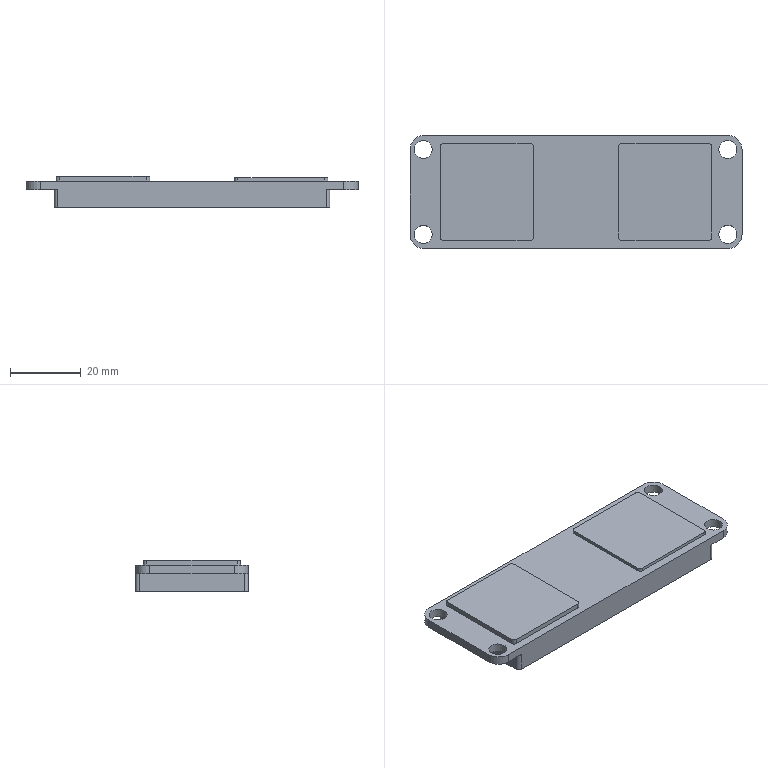NC program | NX | posted with a generic post | part box 94 x 32 x 9 mm
Whole program:
N10 G17 G21 G94 G90
(101_COPY , TOOL : D50-120)
N12 T01 M6
N14 G54
N16 G17 G0 G90 X-97. Y-1.5 S3000 M3
N18 G43 Z49.5 H1
N20 Z6.171
N22 G94 G1 Z5.671 F3000.
N24 X-72.
N26 X72.
N28 X97.
N30 Z6.171
N32 G0 Z49.5
N34 X-97.
N36 Z5.243
N38 G1 Z4.743
N40 X-72.
N42 X72.
N44 X97.
N46 Z5.243
N48 G0 Z49.5
N50 X-97.
N52 Z4.314
N54 G1 Z3.814
N56 X-72.
N58 X72.
N60 X97.
N62 Z4.314
N64 G0 Z49.5
N66 X-97.
N68 Z3.386
N70 G1 Z2.886
N72 X-72.
N74 X72.
N76 X97.
N78 Z3.386
N80 G0 Z49.5
N82 X-97.
N84 Z2.457
N86 G1 Z1.957
N88 X-72.
N90 X72.
N92 X97.
N94 Z2.457
N96 G0 Z49.5
N98 X-97.
N100 Z1.529
N102 G1 Z1.029
N104 X-72.
N106 X72.
N108 X97.
N110 Z1.529
N112 G0 Z49.5
N114 X-97.
N116 Z0.6
N118 G1 Z0.1
N120 X-72.
N122 X72.
N124 X97.
N126 Z0.6
N128 G0 Z49.5
N130 M5
(1013 , TOOL : ER25-D10-20)
N132 T02 M6
N134 G54
N136 G17 G0 G90 X-4.07 Y26. S5000 M3
N138 G43 Z49.5 H2
N140 Z1.7
N142 G94 G1 Z-1.3 F2000.
N144 X-0.713 Y21.
N146 G2 X0. Y19.824 R14.8
N148 X0.713 Y21. R14.8
N150 G1 X4.07 Y26.
N152 Z1.7
N154 G0 Z49.5
N156 Y-26.
N158 Z1.7
N160 G1 Z-1.3
N162 X0.713 Y-21.
N164 G2 X0. Y-19.824 R14.8
N166 G1 X-1.976 Y-15.231
N168 G3 X-1.7 Y-12.75 R11.3
N170 G1 Y12.75
N172 G3 X-1.976 Y15.231 R11.3
N174 X1.976 Y15.231 R5.
N176 X1.7 Y12.75 R11.3
N178 G1 Y-12.75
N180 G3 X1.976 Y-15.231 R11.3
N182 X-1.976 Y-15.231 R5.
N184 G1 X0. Y-19.824
N186 G2 X-0.713 Y-21. R14.8
N188 G1 X-7.77 Y-16.262
N190 G2 X-13. Y-19.05 R6.3
N192 G1 X-37.5
N194 G2 X-43.8 Y-12.75 R6.3
N196 G1 Y12.75
N198 G2 X-37.5 Y19.05 R6.3
N200 G1 X-13.
N202 G2 X-6.7 Y12.75 R6.3
N204 G1 Y-12.75
N206 G2 X-7.77 Y-16.262 R6.3
N208 G1 Z1.7
N210 G0 Z49.5
N212 X1.7 Y-12.75
N214 Z1.7
N216 G1 Z-1.3
N218 X6.7
N220 Y12.75
N222 G2 X13. Y19.05 R6.3
N224 G1 X37.5
N226 G2 X43.8 Y12.75 R6.3
N228 G1 Y-12.75
N230 G2 X37.5 Y-19.05 R6.3
N232 G1 X13.
N234 G2 X6.7 Y-12.75 R6.3
N236 G1 X1.7
N238 Y-26.
N240 Z1.7
N242 G0 Z49.5
N244 M5
(1013_COPY , TOOL : ER25-D10-30_G)
N246 T10 M6
N248 G54
N250 G17 G0 G90 X48.5 Y-11.25 S5000 M3
N252 G43 Z49.5 H10
N254 Z2.5
N256 G94 G1 Z-0.5 F1000.
N258 X43.5
N260 X7.
N262 Y-3.75
N264 X43.5
N266 Y3.75
N268 X7.
N270 Y11.25
N272 X43.5
N274 X48.5
N276 Z2.5
N278 G0 Z49.5
N280 X-2. Y-11.25
N282 Z3.
N284 G1 Z0.
N286 X-7.
N288 X-43.5
N290 Y-3.75
N292 X-7.
N294 Y3.75
N296 X-43.5
N298 Y11.25
N300 X-7.
N302 X-2.
N304 Z3.
N306 G0 Z49.5
(1014 , TOOL : ER25-D10-30_G)
N308 X-1.742 Y33.489
N310 Z1.6
N312 G1 Z-1.4
N314 G2 X0.713 Y21. R9.
N316 G3 X0. Y19.824 R14.8
N318 X-0.713 Y21. R14.8
N320 G2 X1.742 Y33.489 R9.
N322 G1 Z1.6
N324 G0 Z49.5
N326 Y-33.489
N328 Z1.6
N330 G1 Z-1.4
N332 G2 X-0.713 Y-21. R9.
N334 G3 X0. Y-19.824 R14.8
N336 G1 X-1.976 Y-15.231
N338 G3 X-1.7 Y-12.75 R11.3
N340 G1 Y12.75
N342 G3 X-1.976 Y15.231 R11.3
N344 X1.976 Y15.231 R5.
N346 X1.7 Y12.75 R11.3
N348 G1 Y-12.75
N350 G3 X1.976 Y-15.231 R11.3
N352 X-1.976 Y-15.231 R5.
N354 G1 X0. Y-19.824
N356 G3 X0.713 Y-21. R14.8
N358 G1 X7.77 Y-16.262
N360 G2 X6.7 Y-12.75 R6.3
N362 G1 Y12.75
N364 G2 X13. Y19.05 R6.3
N366 G1 X37.5
N368 G2 X43.8 Y12.75 R6.3
N370 G1 Y-12.75
N372 G2 X37.5 Y-19.05 R6.3
N374 G1 X13.
N376 G2 X7.77 Y-16.262 R6.3
N378 G3 X-4.719 Y-13.807 R9.
N380 G1 Y-26.
N382 Z1.6
N384 G0 Z49.5
N386 X-53.047 Y-21.75
N388 Z1.6
N390 G1 Z-1.4
N392 X-52.8
N394 G3 X-43.8 Y-12.75 R9.
N396 G1 Y12.75
N398 G2 X-37.5 Y19.05 R6.3
N400 G1 X-13.
N402 G2 X-6.7 Y12.75 R6.3
N404 G1 Y-12.75
N406 G2 X-13. Y-19.05 R6.3
N408 G1 X-37.5
N410 G2 X-43.8 Y-12.75 R6.3
N412 G3 X-52.8 Y-3.75 R9.
N414 G1 X-57.
N416 Z1.6
N418 G0 Z49.5
(PLANAR_MILL_1_3 , TOOL : ER25-D10-30_G)
N420 X-47.8 Y-2.995
N422 G1 Z-0.9 F4500.
N424 Z-1.4 F1000.
N426 G41 X-47.5 Y-3. D10
N428 X-46.5
N430 G3 X-43.5 Y0. R3.
N432 G1 Y12.75
N434 G2 X-37.5 Y18.75 R6.
N436 G1 X-13.
N438 G2 X-7. Y12.75 R6.
N440 G1 Y-12.75
N442 G2 X-13. Y-18.75 R6.
N444 G1 X-37.5
N446 G2 X-43.5 Y-12.75 R6.
N448 G1 Y0.
N450 Y0.5
N452 G3 X-46.5 Y3.5 R3.
N454 G1 X-47.5
N456 G40
N458 X-47.8 Y3.495
N460 Z-0.9
N462 G0 Z0.5
N464 G1 X28.245 Y-23.05 F6000.
N466 Z-0.9 F4500.
N468 Z-1.4 F1000.
N470 G41 X28.25 Y-22.75
N472 Y-21.75
N474 G3 X25.25 Y-18.75 R3.
N476 G1 X13.
N478 G2 X7. Y-12.75 R6.
N480 G1 Y12.75
N482 G2 X13. Y18.75 R6.
N484 G1 X37.5
N486 G2 X43.5 Y12.75 R6.
N488 G1 Y-12.75
N490 G2 X37.5 Y-18.75 R6.
N492 G1 X25.25
N494 X24.75
N496 G3 X21.75 Y-21.75 R3.
N498 G1 Y-22.75
N500 G40
N502 X21.755 Y-23.05
N504 Z-0.9
N506 G0 Z49.5
N508 M5
(1015 , TOOL : Φ3倒角刀)
N510 T06 M6
N512 G54
N514 G17 G0 G90 X-40.9 Y-0.895 S5000 M3
N516 G43 Z49.5 H6
N518 G94 G1 Z-0.5 F4500.
N520 Z-1. F1000.
N522 G41 X-40.6 Y-0.9 D6
N524 X-40.3
N526 G3 X-39.4 Y0. R0.9
N528 G1 Y12.75
N530 G2 X-37.5 Y14.65 R1.9
N532 G1 X-13.
N534 G2 X-11.1 Y12.75 R1.9
N536 G1 Y-12.75
N538 G2 X-13. Y-14.65 R1.9
N540 G1 X-37.5
N542 G2 X-39.4 Y-12.75 R1.9
N544 G1 Y0.
N546 Y0.5
N548 G3 X-40.3 Y1.4 R0.9
N550 G1 X-40.6
N552 G40
N554 X-40.9 Y1.395
N556 Z-0.5
N558 G0 Z0.5
N560 G1 X26.145 Y-15.65 F6000.
N562 Z-0.5 F4500.
N564 Z-1. F1000.
N566 G41 X26.15 Y-15.35
N568 Y-15.05
N570 G3 X25.25 Y-14.15 R0.9
N572 G1 X13.
N574 G2 X11.6 Y-12.75 R1.4
N576 G1 Y12.75
N578 G2 X13. Y14.15 R1.4
N580 G1 X37.5
N582 G2 X38.9 Y12.75 R1.4
N584 G1 Y-12.75
N586 G2 X37.5 Y-14.15 R1.4
N588 G1 X25.25
N590 X24.75
N592 G3 X23.85 Y-15.05 R0.9
N594 G1 Y-15.35
N596 G40
N598 X23.855 Y-15.65
N600 Z-0.5
N602 G0 Z49.5
(PLANAR_MILL_1_3_COPY_COPY , TOOL : Φ3倒角刀)
N604 X-0.895 Y18.4
N606 G1 Z-1.9 F4500.
N608 Z-2.4 F1000.
N610 G41 X-0.9 Y18.1
N612 Y17.8
N614 G3 X0. Y16.9 R0.9
N616 G1 X43.
N618 G2 X47.9 Y12. R4.9
N620 G1 Y-12.
N622 G2 X43. Y-16.9 R4.9
N624 G1 X-43.
N626 G2 X-47.9 Y-12. R4.9
N628 G1 Y12.
N630 G2 X-43. Y16.9 R4.9
N632 G1 X0.
N634 X0.5
N636 G3 X1.4 Y17.8 R0.9
N638 G1 Y18.1
N640 G40
N642 X1.395 Y18.4
N644 Z-1.9
N646 G0 Z49.5
(PLANAR_MILL_1_3_COPY_COPY_COPY , TOOL : Φ3倒角刀)
N648 X-43.538 Y-11.654
N650 G1 Z-1.9 F4500.
N652 Z-2.4 F1000.
N654 G41 X-44. Y-11.1
N656 G3 X-44.9 Y-12. R0.9
N658 X-43.25 Y-13.65 R1.65
N660 X-44.9 Y-12. R-1.65
N662 X-44.825 Y-12.492 R1.65
N664 X-43.697 Y-13.083 R0.9
N666 G40
N668 G1 X-43.422 Y-12.416
N670 Z-1.9
N672 G0 Z49.5
N674 X-43.538 Y12.346
N676 G1 Z-1.9 F4500.
N678 Z-2.4 F1000.
N680 G41 X-44. Y12.9
N682 G3 X-44.9 Y12. R0.9
N684 X-43.25 Y10.35 R1.65
N686 X-44.9 Y12. R-1.65
N688 X-44.825 Y11.508 R1.65
N690 X-43.697 Y10.917 R0.9
N692 G40
N694 G1 X-43.422 Y11.584
N696 Z-1.9
N698 G0 Z49.5
N700 X42.712 Y12.346
N702 G1 Z-1.9 F4500.
N704 Z-2.4 F1000.
N706 G41 X42.25 Y12.9
N708 G3 X41.35 Y12. R0.9
N710 X43. Y10.35 R1.65
N712 X41.35 Y12. R-1.65
N714 X41.425 Y11.508 R1.65
N716 X42.553 Y10.917 R0.9
N718 G40
N720 G1 X42.828 Y11.584
N722 Z-1.9
N724 G0 Z49.5
N726 X42.712 Y-11.654
N728 G1 Z-1.9 F4500.
N730 Z-2.4 F1000.
N732 G41 X42.25 Y-11.1
N734 G3 X41.35 Y-12. R0.9
N736 X43. Y-13.65 R1.65
N738 X41.35 Y-12. R-1.65
N740 X41.425 Y-12.492 R1.65
N742 X42.553 Y-13.083 R0.9
N744 G40
N746 G1 X42.828 Y-12.416
N748 Z-1.9
N750 G0 Z49.5
N752 M5
N754 M2